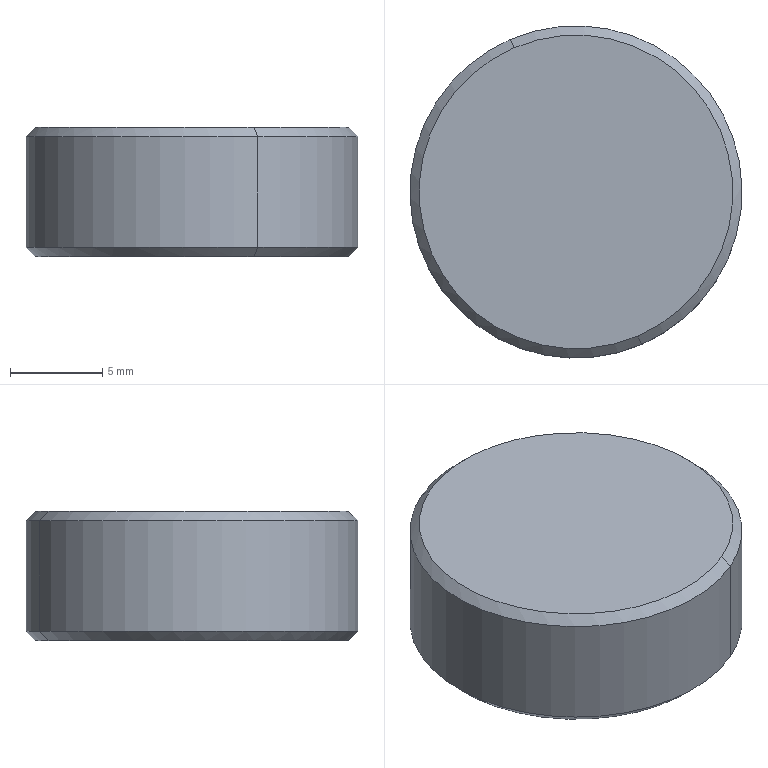Part | SolidWorks | features BaseBody 1 | 1 solid | 21 faces | box 18 x 18 x 7 mm | volume 1609 mm3 | plane 15 | cone 4 | cylinder 2 | commonest cylinder face diameters 18 x2
STEP:
#1=CARTESIAN_POINT('',(289.165,142.694,-47.));
#2=VERTEX_POINT('',#1);
#3=CARTESIAN_POINT('',(282.435,158.306,-47.));
#4=VERTEX_POINT('',#3);
#5=CARTESIAN_POINT('',(285.8,150.5,-47.));
#6=DIRECTION('',(0.,0.,-1.));
#7=DIRECTION('',(0.3959,-0.9183,0.));
#8=AXIS2_PLACEMENT_3D('',#5,#6,#7);
#9=CIRCLE('',#8,8.5);
#10=EDGE_CURVE('',#2,#4,#9,.T.);
#11=ORIENTED_EDGE('',*,*,#10,.F.);
#12=CARTESIAN_POINT('',(289.363,142.235,-46.5));
#13=VERTEX_POINT('',#12);
#14=CARTESIAN_POINT('',(289.165,142.694,-47.));
#15=DIRECTION('',(0.2799,-0.6493,0.7071));
#16=VECTOR('',#15,1000.);
#17=LINE('',#14,#16);
#18=EDGE_CURVE('',#2,#13,#17,.T.);
#19=ORIENTED_EDGE('',*,*,#18,.T.);
#20=CARTESIAN_POINT('',(282.237,158.765,-46.5));
#21=VERTEX_POINT('',#20);
#22=CARTESIAN_POINT('',(285.8,150.5,-46.5));
#23=DIRECTION('',(0.,0.,1.));
#24=DIRECTION('',(0.3959,-0.9183,0.));
#25=AXIS2_PLACEMENT_3D('',#22,#23,#24);
#26=CIRCLE('',#25,9.);
#27=EDGE_CURVE('',#21,#13,#26,.T.);
#28=ORIENTED_EDGE('',*,*,#27,.F.);
#29=CARTESIAN_POINT('',(282.435,158.306,-47.));
#30=DIRECTION('',(-0.2799,0.6493,0.7071));
#31=VECTOR('',#30,1000.);
#32=LINE('',#29,#31);
#33=EDGE_CURVE('',#4,#21,#32,.T.);
#34=ORIENTED_EDGE('',*,*,#33,.F.);
#35=EDGE_LOOP('',(#11,#19,#28,#34));
#36=FACE_OUTER_BOUND('',#35,.T.);
#37=CARTESIAN_POINT('',(285.8,150.5,-47.));
#38=DIRECTION('',(0.,0.,1.));
#39=DIRECTION('',(-0.3959,0.9183,0.));
#40=AXIS2_PLACEMENT_3D('',#37,#38,#39);
#41=CONICAL_SURFACE('',#40,8.5,0.7854);
#42=ADVANCED_FACE('',(#36),#41,.T.);
#43=CARTESIAN_POINT('',(282.435,158.306,-40.));
#44=VERTEX_POINT('',#43);
#45=CARTESIAN_POINT('',(289.165,142.694,-40.));
#46=VERTEX_POINT('',#45);
#47=CARTESIAN_POINT('',(285.8,150.5,-40.));
#48=DIRECTION('',(0.,0.,1.));
#49=DIRECTION('',(0.3959,-0.9183,0.));
#50=AXIS2_PLACEMENT_3D('',#47,#48,#49);
#51=CIRCLE('',#50,8.5);
#52=EDGE_CURVE('',#44,#46,#51,.T.);
#53=ORIENTED_EDGE('',*,*,#52,.F.);
#54=CARTESIAN_POINT('',(282.237,158.765,-40.5));
#55=VERTEX_POINT('',#54);
#56=CARTESIAN_POINT('',(282.237,158.765,-40.5));
#57=DIRECTION('',(-0.2799,0.6493,-0.7071));
#58=VECTOR('',#57,1000.);
#59=LINE('',#56,#58);
#60=EDGE_CURVE('',#44,#55,#59,.T.);
#61=ORIENTED_EDGE('',*,*,#60,.T.);
#62=CARTESIAN_POINT('',(289.363,142.235,-40.5));
#63=VERTEX_POINT('',#62);
#64=CARTESIAN_POINT('',(285.8,150.5,-40.5));
#65=DIRECTION('',(0.,0.,-1.));
#66=DIRECTION('',(0.3959,-0.9183,0.));
#67=AXIS2_PLACEMENT_3D('',#64,#65,#66);
#68=CIRCLE('',#67,9.);
#69=EDGE_CURVE('',#63,#55,#68,.T.);
#70=ORIENTED_EDGE('',*,*,#69,.F.);
#71=CARTESIAN_POINT('',(289.363,142.235,-40.5));
#72=DIRECTION('',(0.2799,-0.6493,-0.7071));
#73=VECTOR('',#72,1000.);
#74=LINE('',#71,#73);
#75=EDGE_CURVE('',#46,#63,#74,.T.);
#76=ORIENTED_EDGE('',*,*,#75,.F.);
#77=EDGE_LOOP('',(#53,#61,#70,#76));
#78=FACE_OUTER_BOUND('',#77,.T.);
#79=CARTESIAN_POINT('',(285.8,150.5,-40.5));
#80=DIRECTION('',(0.,0.,-1.));
#81=DIRECTION('',(0.3959,-0.9183,0.));
#82=AXIS2_PLACEMENT_3D('',#79,#80,#81);
#83=CONICAL_SURFACE('',#82,9.,0.7854);
#84=ADVANCED_FACE('',(#78),#83,.T.);
#85=ORIENTED_EDGE('',*,*,#69,.T.);
#86=CARTESIAN_POINT('',(282.237,158.765,-40.));
#87=DIRECTION('',(0.,0.,-1.));
#88=VECTOR('',#87,1000.);
#89=LINE('',#86,#88);
#90=EDGE_CURVE('',#55,#21,#89,.T.);
#91=ORIENTED_EDGE('',*,*,#90,.T.);
#92=ORIENTED_EDGE('',*,*,#27,.T.);
#93=CARTESIAN_POINT('',(289.363,142.235,-40.));
#94=DIRECTION('',(0.,0.,-1.));
#95=VECTOR('',#94,1000.);
#96=LINE('',#93,#95);
#97=EDGE_CURVE('',#63,#13,#96,.T.);
#98=ORIENTED_EDGE('',*,*,#97,.F.);
#99=EDGE_LOOP('',(#85,#91,#92,#98));
#100=FACE_OUTER_BOUND('',#99,.T.);
#101=CARTESIAN_POINT('',(285.8,150.5,-40.));
#102=DIRECTION('',(0.,0.,-1.));
#103=DIRECTION('',(0.3959,-0.9183,0.));
#104=AXIS2_PLACEMENT_3D('',#101,#102,#103);
#105=CYLINDRICAL_SURFACE('',#104,9.);
#106=ADVANCED_FACE('',(#100),#105,.T.);
#107=ORIENTED_EDGE('',*,*,#90,.F.);
#108=CARTESIAN_POINT('',(285.8,150.5,-40.5));
#109=DIRECTION('',(0.,0.,-1.));
#110=DIRECTION('',(0.3959,-0.9183,0.));
#111=AXIS2_PLACEMENT_3D('',#108,#109,#110);
#112=CIRCLE('',#111,9.);
#113=EDGE_CURVE('',#55,#63,#112,.T.);
#114=ORIENTED_EDGE('',*,*,#113,.T.);
#115=ORIENTED_EDGE('',*,*,#97,.T.);
#116=CARTESIAN_POINT('',(285.8,150.5,-46.5));
#117=DIRECTION('',(0.,0.,1.));
#118=DIRECTION('',(0.3959,-0.9183,0.));
#119=AXIS2_PLACEMENT_3D('',#116,#117,#118);
#120=CIRCLE('',#119,9.);
#121=EDGE_CURVE('',#13,#21,#120,.T.);
#122=ORIENTED_EDGE('',*,*,#121,.T.);
#123=EDGE_LOOP('',(#107,#114,#115,#122));
#124=FACE_OUTER_BOUND('',#123,.T.);
#125=CARTESIAN_POINT('',(285.8,150.5,-40.));
#126=DIRECTION('',(0.,0.,-1.));
#127=DIRECTION('',(0.3959,-0.9183,0.));
#128=AXIS2_PLACEMENT_3D('',#125,#126,#127);
#129=CYLINDRICAL_SURFACE('',#128,9.);
#130=ADVANCED_FACE('',(#124),#129,.T.);
#131=CARTESIAN_POINT('',(285.8,150.5,-40.));
#132=DIRECTION('',(0.,0.,1.));
#133=DIRECTION('',(0.3959,-0.9183,0.));
#134=AXIS2_PLACEMENT_3D('',#131,#132,#133);
#135=CIRCLE('',#134,8.5);
#136=EDGE_CURVE('',#46,#44,#135,.T.);
#137=ORIENTED_EDGE('',*,*,#136,.T.);
#138=ORIENTED_EDGE('',*,*,#52,.T.);
#139=EDGE_LOOP('',(#137,#138));
#140=FACE_OUTER_BOUND('',#139,.T.);
#141=CARTESIAN_POINT('',(285.8,150.5,-40.));
#142=DIRECTION('',(0.,0.,-1.));
#143=DIRECTION('',(0.3959,-0.9183,0.));
#144=AXIS2_PLACEMENT_3D('',#141,#142,#143);
#145=PLANE('',#144);
#146=ADVANCED_FACE('',(#140),#145,.F.);
#147=CARTESIAN_POINT('',(282.559,152.914,-47.));
#148=VERTEX_POINT('',#147);
#149=CARTESIAN_POINT('',(282.089,148.9,-47.));
#150=VERTEX_POINT('',#149);
#151=CARTESIAN_POINT('',(282.122,149.187,-47.));
#152=DIRECTION('',(-0.1163,-0.9932,0.));
#153=VECTOR('',#152,1000.);
#154=LINE('',#151,#153);
#155=EDGE_CURVE('',#148,#150,#154,.T.);
#156=ORIENTED_EDGE('',*,*,#155,.T.);
#157=CARTESIAN_POINT('',(285.33,146.486,-47.));
#158=VERTEX_POINT('',#157);
#159=CARTESIAN_POINT('',(285.098,146.658,-47.));
#160=DIRECTION('',(0.802,-0.5973,0.));
#161=VECTOR('',#160,1000.);
#162=LINE('',#159,#161);
#163=EDGE_CURVE('',#150,#158,#162,.T.);
#164=ORIENTED_EDGE('',*,*,#163,.T.);
#165=CARTESIAN_POINT('',(289.041,148.086,-47.));
#166=VERTEX_POINT('',#165);
#167=CARTESIAN_POINT('',(288.776,147.972,-47.));
#168=DIRECTION('',(0.9183,0.3959,0.));
#169=VECTOR('',#168,1000.);
#170=LINE('',#167,#169);
#171=EDGE_CURVE('',#158,#166,#170,.T.);
#172=ORIENTED_EDGE('',*,*,#171,.T.);
#173=CARTESIAN_POINT('',(289.511,152.1,-47.));
#174=VERTEX_POINT('',#173);
#175=CARTESIAN_POINT('',(289.478,151.813,-47.));
#176=DIRECTION('',(0.1163,0.9932,0.));
#177=VECTOR('',#176,1000.);
#178=LINE('',#175,#177);
#179=EDGE_CURVE('',#166,#174,#178,.T.);
#180=ORIENTED_EDGE('',*,*,#179,.T.);
#181=CARTESIAN_POINT('',(286.27,154.514,-47.));
#182=VERTEX_POINT('',#181);
#183=CARTESIAN_POINT('',(286.502,154.342,-47.));
#184=DIRECTION('',(-0.802,0.5973,0.));
#185=VECTOR('',#184,1000.);
#186=LINE('',#183,#185);
#187=EDGE_CURVE('',#174,#182,#186,.T.);
#188=ORIENTED_EDGE('',*,*,#187,.T.);
#189=CARTESIAN_POINT('',(282.824,153.028,-47.));
#190=DIRECTION('',(-0.9183,-0.3959,0.));
#191=VECTOR('',#190,1000.);
#192=LINE('',#189,#191);
#193=EDGE_CURVE('',#182,#148,#192,.T.);
#194=ORIENTED_EDGE('',*,*,#193,.T.);
#195=EDGE_LOOP('',(#156,#164,#172,#180,#188,#194));
#196=FACE_BOUND('',#195,.T.);
#197=CARTESIAN_POINT('',(285.8,150.5,-47.));
#198=DIRECTION('',(0.,0.,-1.));
#199=DIRECTION('',(0.3959,-0.9183,0.));
#200=AXIS2_PLACEMENT_3D('',#197,#198,#199);
#201=CIRCLE('',#200,8.5);
#202=EDGE_CURVE('',#4,#2,#201,.T.);
#203=ORIENTED_EDGE('',*,*,#202,.T.);
#204=ORIENTED_EDGE('',*,*,#10,.T.);
#205=EDGE_LOOP('',(#203,#204));
#206=FACE_OUTER_BOUND('',#205,.T.);
#207=CARTESIAN_POINT('',(285.8,150.5,-47.));
#208=DIRECTION('',(0.,0.,-1.));
#209=DIRECTION('',(0.3959,-0.9183,0.));
#210=AXIS2_PLACEMENT_3D('',#207,#208,#209);
#211=PLANE('',#210);
#212=ADVANCED_FACE('',(#196,#206),#211,.T.);
#213=ORIENTED_EDGE('',*,*,#60,.F.);
#214=ORIENTED_EDGE('',*,*,#136,.F.);
#215=ORIENTED_EDGE('',*,*,#75,.T.);
#216=ORIENTED_EDGE('',*,*,#113,.F.);
#217=EDGE_LOOP('',(#213,#214,#215,#216));
#218=FACE_OUTER_BOUND('',#217,.T.);
#219=CARTESIAN_POINT('',(285.8,150.5,-40.5));
#220=DIRECTION('',(0.,0.,-1.));
#221=DIRECTION('',(0.3959,-0.9183,0.));
#222=AXIS2_PLACEMENT_3D('',#219,#220,#221);
#223=CONICAL_SURFACE('',#222,9.,0.7854);
#224=ADVANCED_FACE('',(#218),#223,.T.);
#225=ORIENTED_EDGE('',*,*,#18,.F.);
#226=ORIENTED_EDGE('',*,*,#202,.F.);
#227=ORIENTED_EDGE('',*,*,#33,.T.);
#228=ORIENTED_EDGE('',*,*,#121,.F.);
#229=EDGE_LOOP('',(#225,#226,#227,#228));
#230=FACE_OUTER_BOUND('',#229,.T.);
#231=CARTESIAN_POINT('',(285.8,150.5,-47.));
#232=DIRECTION('',(0.,0.,1.));
#233=DIRECTION('',(-0.3959,0.9183,0.));
#234=AXIS2_PLACEMENT_3D('',#231,#232,#233);
#235=CONICAL_SURFACE('',#234,8.5,0.7854);
#236=ADVANCED_FACE('',(#230),#235,.T.);
#237=CARTESIAN_POINT('',(286.203,153.941,-42.));
#238=VERTEX_POINT('',#237);
#239=CARTESIAN_POINT('',(286.203,153.941,-46.5));
#240=VERTEX_POINT('',#239);
#241=CARTESIAN_POINT('',(286.203,153.941,-42.));
#242=DIRECTION('',(0.,0.,-1.));
#243=VECTOR('',#242,1000.);
#244=LINE('',#241,#243);
#245=EDGE_CURVE('',#238,#240,#244,.T.);
#246=ORIENTED_EDGE('',*,*,#245,.T.);
#247=CARTESIAN_POINT('',(288.981,151.871,-46.5));
#248=VERTEX_POINT('',#247);
#249=CARTESIAN_POINT('',(288.981,151.871,-46.5));
#250=DIRECTION('',(0.802,-0.5973,0.));
#251=VECTOR('',#250,1000.);
#252=LINE('',#249,#251);
#253=EDGE_CURVE('',#240,#248,#252,.T.);
#254=ORIENTED_EDGE('',*,*,#253,.T.);
#255=CARTESIAN_POINT('',(288.981,151.871,-42.));
#256=VERTEX_POINT('',#255);
#257=CARTESIAN_POINT('',(288.981,151.871,-42.));
#258=DIRECTION('',(0.,0.,-1.));
#259=VECTOR('',#258,1000.);
#260=LINE('',#257,#259);
#261=EDGE_CURVE('',#256,#248,#260,.T.);
#262=ORIENTED_EDGE('',*,*,#261,.F.);
#263=CARTESIAN_POINT('',(286.203,153.941,-42.));
#264=DIRECTION('',(0.802,-0.5973,0.));
#265=VECTOR('',#264,1000.);
#266=LINE('',#263,#265);
#267=EDGE_CURVE('',#238,#256,#266,.T.);
#268=ORIENTED_EDGE('',*,*,#267,.F.);
#269=EDGE_LOOP('',(#246,#254,#262,#268));
#270=FACE_OUTER_BOUND('',#269,.T.);
#271=CARTESIAN_POINT('',(286.203,153.941,-42.));
#272=DIRECTION('',(0.5973,0.802,0.));
#273=DIRECTION('',(0.802,-0.5973,0.));
#274=AXIS2_PLACEMENT_3D('',#271,#272,#273);
#275=PLANE('',#274);
#276=ADVANCED_FACE('',(#270),#275,.F.);
#277=CARTESIAN_POINT('',(283.022,152.569,-42.));
#278=VERTEX_POINT('',#277);
#279=CARTESIAN_POINT('',(283.022,152.569,-46.5));
#280=VERTEX_POINT('',#279);
#281=CARTESIAN_POINT('',(283.022,152.569,-42.));
#282=DIRECTION('',(0.,0.,-1.));
#283=VECTOR('',#282,1000.);
#284=LINE('',#281,#283);
#285=EDGE_CURVE('',#278,#280,#284,.T.);
#286=ORIENTED_EDGE('',*,*,#285,.T.);
#287=CARTESIAN_POINT('',(286.203,153.941,-46.5));
#288=DIRECTION('',(0.9183,0.3959,0.));
#289=VECTOR('',#288,1000.);
#290=LINE('',#287,#289);
#291=EDGE_CURVE('',#280,#240,#290,.T.);
#292=ORIENTED_EDGE('',*,*,#291,.T.);
#293=ORIENTED_EDGE('',*,*,#245,.F.);
#294=CARTESIAN_POINT('',(283.022,152.569,-42.));
#295=DIRECTION('',(0.9183,0.3959,0.));
#296=VECTOR('',#295,1000.);
#297=LINE('',#294,#296);
#298=EDGE_CURVE('',#278,#238,#297,.T.);
#299=ORIENTED_EDGE('',*,*,#298,.F.);
#300=EDGE_LOOP('',(#286,#292,#293,#299));
#301=FACE_OUTER_BOUND('',#300,.T.);
#302=CARTESIAN_POINT('',(283.022,152.569,-42.));
#303=DIRECTION('',(-0.3959,0.9183,0.));
#304=DIRECTION('',(0.9183,0.3959,0.));
#305=AXIS2_PLACEMENT_3D('',#302,#303,#304);
#306=PLANE('',#305);
#307=ADVANCED_FACE('',(#301),#306,.F.);
#308=CARTESIAN_POINT('',(282.619,149.129,-42.));
#309=VERTEX_POINT('',#308);
#310=CARTESIAN_POINT('',(282.619,149.129,-46.5));
#311=VERTEX_POINT('',#310);
#312=CARTESIAN_POINT('',(282.619,149.129,-42.));
#313=DIRECTION('',(0.,0.,-1.));
#314=VECTOR('',#313,1000.);
#315=LINE('',#312,#314);
#316=EDGE_CURVE('',#309,#311,#315,.T.);
#317=ORIENTED_EDGE('',*,*,#316,.T.);
#318=CARTESIAN_POINT('',(283.022,152.569,-46.5));
#319=DIRECTION('',(0.1163,0.9932,0.));
#320=VECTOR('',#319,1000.);
#321=LINE('',#318,#320);
#322=EDGE_CURVE('',#311,#280,#321,.T.);
#323=ORIENTED_EDGE('',*,*,#322,.T.);
#324=ORIENTED_EDGE('',*,*,#285,.F.);
#325=CARTESIAN_POINT('',(282.619,149.129,-42.));
#326=DIRECTION('',(0.1163,0.9932,0.));
#327=VECTOR('',#326,1000.);
#328=LINE('',#325,#327);
#329=EDGE_CURVE('',#309,#278,#328,.T.);
#330=ORIENTED_EDGE('',*,*,#329,.F.);
#331=EDGE_LOOP('',(#317,#323,#324,#330));
#332=FACE_OUTER_BOUND('',#331,.T.);
#333=CARTESIAN_POINT('',(282.619,149.129,-42.));
#334=DIRECTION('',(-0.9932,0.1163,0.));
#335=DIRECTION('',(0.1163,0.9932,0.));
#336=AXIS2_PLACEMENT_3D('',#333,#334,#335);
#337=PLANE('',#336);
#338=ADVANCED_FACE('',(#332),#337,.F.);
#339=CARTESIAN_POINT('',(285.397,147.059,-42.));
#340=VERTEX_POINT('',#339);
#341=CARTESIAN_POINT('',(285.397,147.059,-46.5));
#342=VERTEX_POINT('',#341);
#343=CARTESIAN_POINT('',(285.397,147.059,-42.));
#344=DIRECTION('',(0.,0.,-1.));
#345=VECTOR('',#344,1000.);
#346=LINE('',#343,#345);
#347=EDGE_CURVE('',#340,#342,#346,.T.);
#348=ORIENTED_EDGE('',*,*,#347,.T.);
#349=CARTESIAN_POINT('',(282.619,149.129,-46.5));
#350=DIRECTION('',(-0.802,0.5973,0.));
#351=VECTOR('',#350,1000.);
#352=LINE('',#349,#351);
#353=EDGE_CURVE('',#342,#311,#352,.T.);
#354=ORIENTED_EDGE('',*,*,#353,.T.);
#355=ORIENTED_EDGE('',*,*,#316,.F.);
#356=CARTESIAN_POINT('',(285.397,147.059,-42.));
#357=DIRECTION('',(-0.802,0.5973,0.));
#358=VECTOR('',#357,1000.);
#359=LINE('',#356,#358);
#360=EDGE_CURVE('',#340,#309,#359,.T.);
#361=ORIENTED_EDGE('',*,*,#360,.F.);
#362=EDGE_LOOP('',(#348,#354,#355,#361));
#363=FACE_OUTER_BOUND('',#362,.T.);
#364=CARTESIAN_POINT('',(285.397,147.059,-42.));
#365=DIRECTION('',(-0.5973,-0.802,0.));
#366=DIRECTION('',(-0.802,0.5973,0.));
#367=AXIS2_PLACEMENT_3D('',#364,#365,#366);
#368=PLANE('',#367);
#369=ADVANCED_FACE('',(#363),#368,.F.);
#370=CARTESIAN_POINT('',(288.578,148.431,-42.));
#371=VERTEX_POINT('',#370);
#372=CARTESIAN_POINT('',(288.578,148.431,-46.5));
#373=VERTEX_POINT('',#372);
#374=CARTESIAN_POINT('',(288.578,148.431,-42.));
#375=DIRECTION('',(0.,0.,-1.));
#376=VECTOR('',#375,1000.);
#377=LINE('',#374,#376);
#378=EDGE_CURVE('',#371,#373,#377,.T.);
#379=ORIENTED_EDGE('',*,*,#378,.T.);
#380=CARTESIAN_POINT('',(285.397,147.059,-46.5));
#381=DIRECTION('',(-0.9183,-0.3959,0.));
#382=VECTOR('',#381,1000.);
#383=LINE('',#380,#382);
#384=EDGE_CURVE('',#373,#342,#383,.T.);
#385=ORIENTED_EDGE('',*,*,#384,.T.);
#386=ORIENTED_EDGE('',*,*,#347,.F.);
#387=CARTESIAN_POINT('',(288.578,148.431,-42.));
#388=DIRECTION('',(-0.9183,-0.3959,0.));
#389=VECTOR('',#388,1000.);
#390=LINE('',#387,#389);
#391=EDGE_CURVE('',#371,#340,#390,.T.);
#392=ORIENTED_EDGE('',*,*,#391,.F.);
#393=EDGE_LOOP('',(#379,#385,#386,#392));
#394=FACE_OUTER_BOUND('',#393,.T.);
#395=CARTESIAN_POINT('',(288.578,148.431,-42.));
#396=DIRECTION('',(0.3959,-0.9183,0.));
#397=DIRECTION('',(-0.9183,-0.3959,0.));
#398=AXIS2_PLACEMENT_3D('',#395,#396,#397);
#399=PLANE('',#398);
#400=ADVANCED_FACE('',(#394),#399,.F.);
#401=ORIENTED_EDGE('',*,*,#261,.T.);
#402=CARTESIAN_POINT('',(288.578,148.431,-46.5));
#403=DIRECTION('',(-0.1163,-0.9932,0.));
#404=VECTOR('',#403,1000.);
#405=LINE('',#402,#404);
#406=EDGE_CURVE('',#248,#373,#405,.T.);
#407=ORIENTED_EDGE('',*,*,#406,.T.);
#408=ORIENTED_EDGE('',*,*,#378,.F.);
#409=CARTESIAN_POINT('',(288.981,151.871,-42.));
#410=DIRECTION('',(-0.1163,-0.9932,0.));
#411=VECTOR('',#410,1000.);
#412=LINE('',#409,#411);
#413=EDGE_CURVE('',#256,#371,#412,.T.);
#414=ORIENTED_EDGE('',*,*,#413,.F.);
#415=EDGE_LOOP('',(#401,#407,#408,#414));
#416=FACE_OUTER_BOUND('',#415,.T.);
#417=CARTESIAN_POINT('',(288.981,151.871,-42.));
#418=DIRECTION('',(0.9932,-0.1163,0.));
#419=DIRECTION('',(-0.1163,-0.9932,0.));
#420=AXIS2_PLACEMENT_3D('',#417,#418,#419);
#421=PLANE('',#420);
#422=ADVANCED_FACE('',(#416),#421,.F.);
#423=ORIENTED_EDGE('',*,*,#267,.T.);
#424=ORIENTED_EDGE('',*,*,#413,.T.);
#425=ORIENTED_EDGE('',*,*,#391,.T.);
#426=ORIENTED_EDGE('',*,*,#360,.T.);
#427=ORIENTED_EDGE('',*,*,#329,.T.);
#428=ORIENTED_EDGE('',*,*,#298,.T.);
#429=EDGE_LOOP('',(#423,#424,#425,#426,#427,#428));
#430=FACE_OUTER_BOUND('',#429,.T.);
#431=CARTESIAN_POINT('',(288.981,151.871,-42.));
#432=DIRECTION('',(0.,0.,-1.));
#433=DIRECTION('',(0.3959,-0.9183,0.));
#434=AXIS2_PLACEMENT_3D('',#431,#432,#433);
#435=PLANE('',#434);
#436=ADVANCED_FACE('',(#430),#435,.T.);
#437=CARTESIAN_POINT('',(286.203,153.941,-46.5));
#438=DIRECTION('',(-0.08793,-0.7508,0.6547));
#439=VECTOR('',#438,1000.);
#440=LINE('',#437,#439);
#441=EDGE_CURVE('',#182,#240,#440,.T.);
#442=ORIENTED_EDGE('',*,*,#441,.F.);
#443=ORIENTED_EDGE('',*,*,#187,.F.);
#444=CARTESIAN_POINT('',(288.981,151.871,-46.5));
#445=DIRECTION('',(0.6942,0.2993,-0.6547));
#446=VECTOR('',#445,1000.);
#447=LINE('',#444,#446);
#448=EDGE_CURVE('',#248,#174,#447,.T.);
#449=ORIENTED_EDGE('',*,*,#448,.F.);
#450=ORIENTED_EDGE('',*,*,#253,.F.);
#451=EDGE_LOOP('',(#442,#443,#449,#450));
#452=FACE_OUTER_BOUND('',#451,.T.);
#453=CARTESIAN_POINT('',(286.203,153.941,-46.5));
#454=DIRECTION('',(-0.4224,-0.5671,-0.7071));
#455=DIRECTION('',(0.6942,0.2993,-0.6547));
#456=AXIS2_PLACEMENT_3D('',#453,#454,#455);
#457=PLANE('',#456);
#458=ADVANCED_FACE('',(#452),#457,.T.);
#459=ORIENTED_EDGE('',*,*,#448,.T.);
#460=ORIENTED_EDGE('',*,*,#179,.F.);
#461=CARTESIAN_POINT('',(288.578,148.431,-46.5));
#462=DIRECTION('',(0.6062,-0.4515,-0.6547));
#463=VECTOR('',#462,1000.);
#464=LINE('',#461,#463);
#465=EDGE_CURVE('',#373,#166,#464,.T.);
#466=ORIENTED_EDGE('',*,*,#465,.F.);
#467=ORIENTED_EDGE('',*,*,#406,.F.);
#468=EDGE_LOOP('',(#459,#460,#466,#467));
#469=FACE_OUTER_BOUND('',#468,.T.);
#470=CARTESIAN_POINT('',(288.981,151.871,-46.5));
#471=DIRECTION('',(-0.7023,0.08225,-0.7071));
#472=DIRECTION('',(0.6942,0.2993,-0.6547));
#473=AXIS2_PLACEMENT_3D('',#470,#471,#472);
#474=PLANE('',#473);
#475=ADVANCED_FACE('',(#469),#474,.T.);
#476=ORIENTED_EDGE('',*,*,#441,.T.);
#477=ORIENTED_EDGE('',*,*,#291,.F.);
#478=CARTESIAN_POINT('',(283.022,152.569,-46.5));
#479=DIRECTION('',(0.6062,-0.4515,0.6547));
#480=VECTOR('',#479,1000.);
#481=LINE('',#478,#480);
#482=EDGE_CURVE('',#148,#280,#481,.T.);
#483=ORIENTED_EDGE('',*,*,#482,.F.);
#484=ORIENTED_EDGE('',*,*,#193,.F.);
#485=EDGE_LOOP('',(#476,#477,#483,#484));
#486=FACE_OUTER_BOUND('',#485,.T.);
#487=CARTESIAN_POINT('',(283.022,152.569,-46.5));
#488=DIRECTION('',(0.2799,-0.6493,-0.7071));
#489=DIRECTION('',(0.2799,-0.6493,0.7071));
#490=AXIS2_PLACEMENT_3D('',#487,#488,#489);
#491=PLANE('',#490);
#492=ADVANCED_FACE('',(#486),#491,.T.);
#493=ORIENTED_EDGE('',*,*,#465,.T.);
#494=ORIENTED_EDGE('',*,*,#171,.F.);
#495=CARTESIAN_POINT('',(285.397,147.059,-46.5));
#496=DIRECTION('',(-0.08793,-0.7508,-0.6547));
#497=VECTOR('',#496,1000.);
#498=LINE('',#495,#497);
#499=EDGE_CURVE('',#342,#158,#498,.T.);
#500=ORIENTED_EDGE('',*,*,#499,.F.);
#501=ORIENTED_EDGE('',*,*,#384,.F.);
#502=EDGE_LOOP('',(#493,#494,#500,#501));
#503=FACE_OUTER_BOUND('',#502,.T.);
#504=CARTESIAN_POINT('',(288.578,148.431,-46.5));
#505=DIRECTION('',(-0.2799,0.6493,-0.7071));
#506=DIRECTION('',(0.2799,-0.6493,-0.7071));
#507=AXIS2_PLACEMENT_3D('',#504,#505,#506);
#508=PLANE('',#507);
#509=ADVANCED_FACE('',(#503),#508,.T.);
#510=ORIENTED_EDGE('',*,*,#482,.T.);
#511=ORIENTED_EDGE('',*,*,#322,.F.);
#512=CARTESIAN_POINT('',(283.528,149.52,-45.643));
#513=DIRECTION('',(0.6942,0.2993,0.6547));
#514=VECTOR('',#513,1000.);
#515=LINE('',#512,#514);
#516=EDGE_CURVE('',#150,#311,#515,.T.);
#517=ORIENTED_EDGE('',*,*,#516,.F.);
#518=ORIENTED_EDGE('',*,*,#155,.F.);
#519=EDGE_LOOP('',(#510,#511,#517,#518));
#520=FACE_OUTER_BOUND('',#519,.T.);
#521=CARTESIAN_POINT('',(282.619,149.129,-46.5));
#522=DIRECTION('',(0.7023,-0.08225,-0.7071));
#523=DIRECTION('',(0.6942,0.2993,0.6547));
#524=AXIS2_PLACEMENT_3D('',#521,#522,#523);
#525=PLANE('',#524);
#526=ADVANCED_FACE('',(#520),#525,.T.);
#527=ORIENTED_EDGE('',*,*,#499,.T.);
#528=ORIENTED_EDGE('',*,*,#163,.F.);
#529=ORIENTED_EDGE('',*,*,#516,.T.);
#530=ORIENTED_EDGE('',*,*,#353,.F.);
#531=EDGE_LOOP('',(#527,#528,#529,#530));
#532=FACE_OUTER_BOUND('',#531,.T.);
#533=CARTESIAN_POINT('',(285.397,147.059,-46.5));
#534=DIRECTION('',(0.4224,0.5671,-0.7071));
#535=DIRECTION('',(0.6942,0.2993,0.6547));
#536=AXIS2_PLACEMENT_3D('',#533,#534,#535);
#537=PLANE('',#536);
#538=ADVANCED_FACE('',(#532),#537,.T.);
#539=CLOSED_SHELL('',(#42,#84,#106,#130,#146,#212,#224,#236,#276,#307,#338,#369,#400,#422,#436,#458,#475,#492,#509,#526,#538));
#540=MANIFOLD_SOLID_BREP('',#539);
#541=CARTESIAN_POINT('',(0.,0.,0.));
#542=DIRECTION('',(0.,0.,1.));
#543=DIRECTION('',(1.,0.,0.));
#544=AXIS2_PLACEMENT_3D('',#541,#542,#543);
#545=(LENGTH_UNIT()NAMED_UNIT(*)SI_UNIT(.MILLI.,.METRE.));
#546=UNCERTAINTY_MEASURE_WITH_UNIT(LENGTH_MEASURE(0.00001),#545,'','');
#547=(NAMED_UNIT(*)PLANE_ANGLE_UNIT()SI_UNIT($,.RADIAN.));
#548=(NAMED_UNIT(*)SI_UNIT($,.STERADIAN.)SOLID_ANGLE_UNIT());
#549=(GEOMETRIC_REPRESENTATION_CONTEXT(3)GLOBAL_UNCERTAINTY_ASSIGNED_CONTEXT((#546))GLOBAL_UNIT_ASSIGNED_CONTEXT((#545,#547,#548))REPRESENTATION_CONTEXT('',''));
#550=ADVANCED_BREP_SHAPE_REPRESENTATION('',(#540,#544),#549);